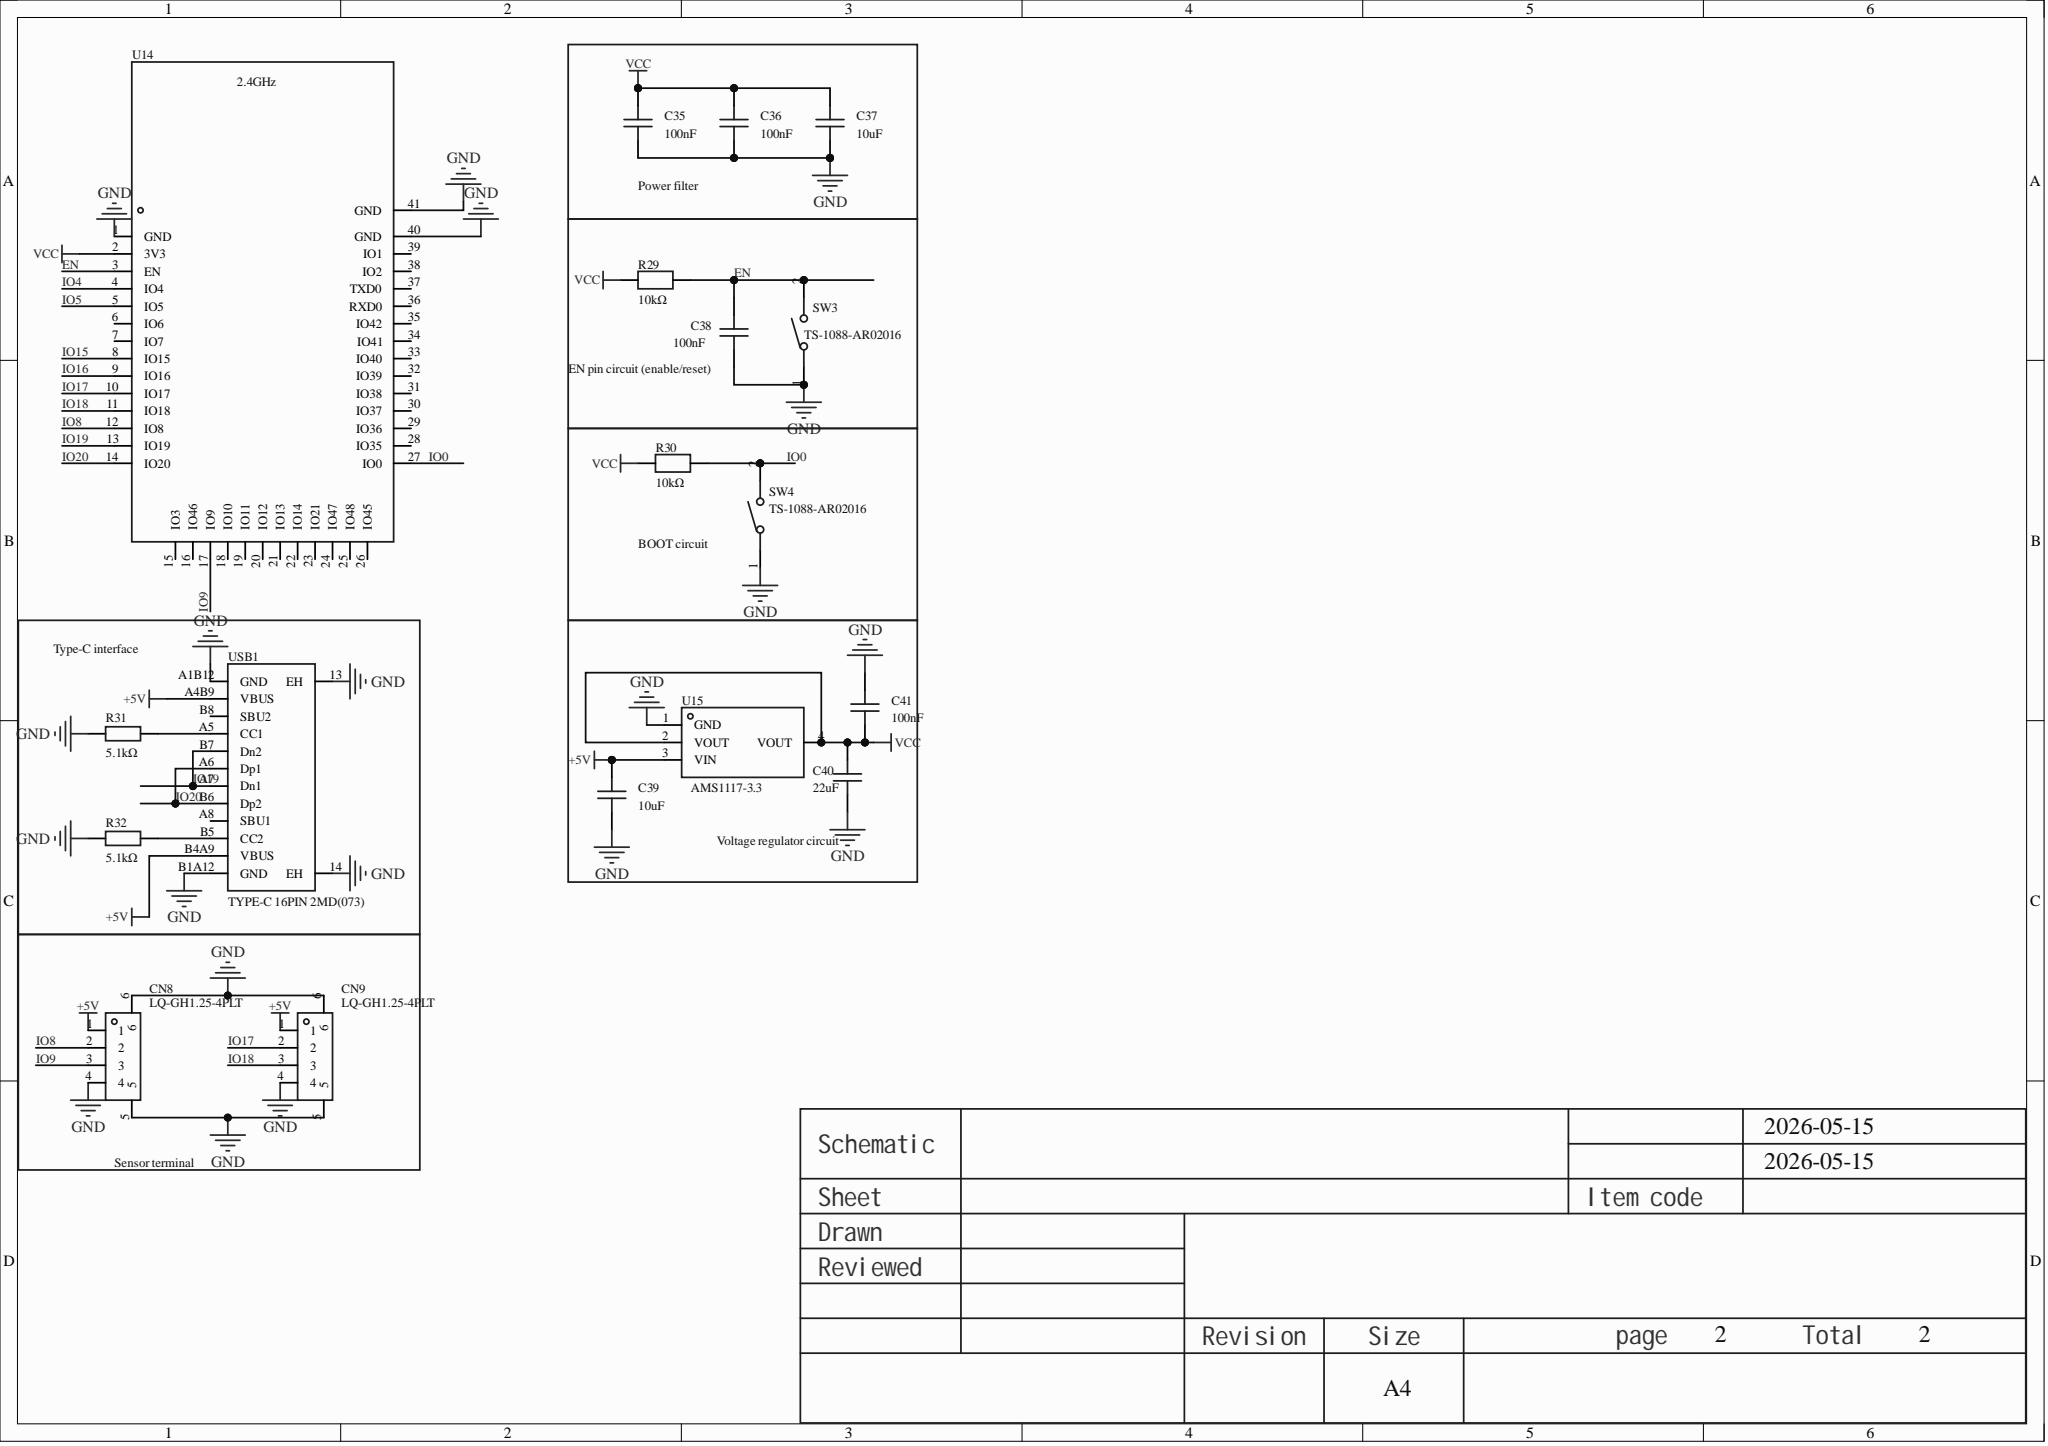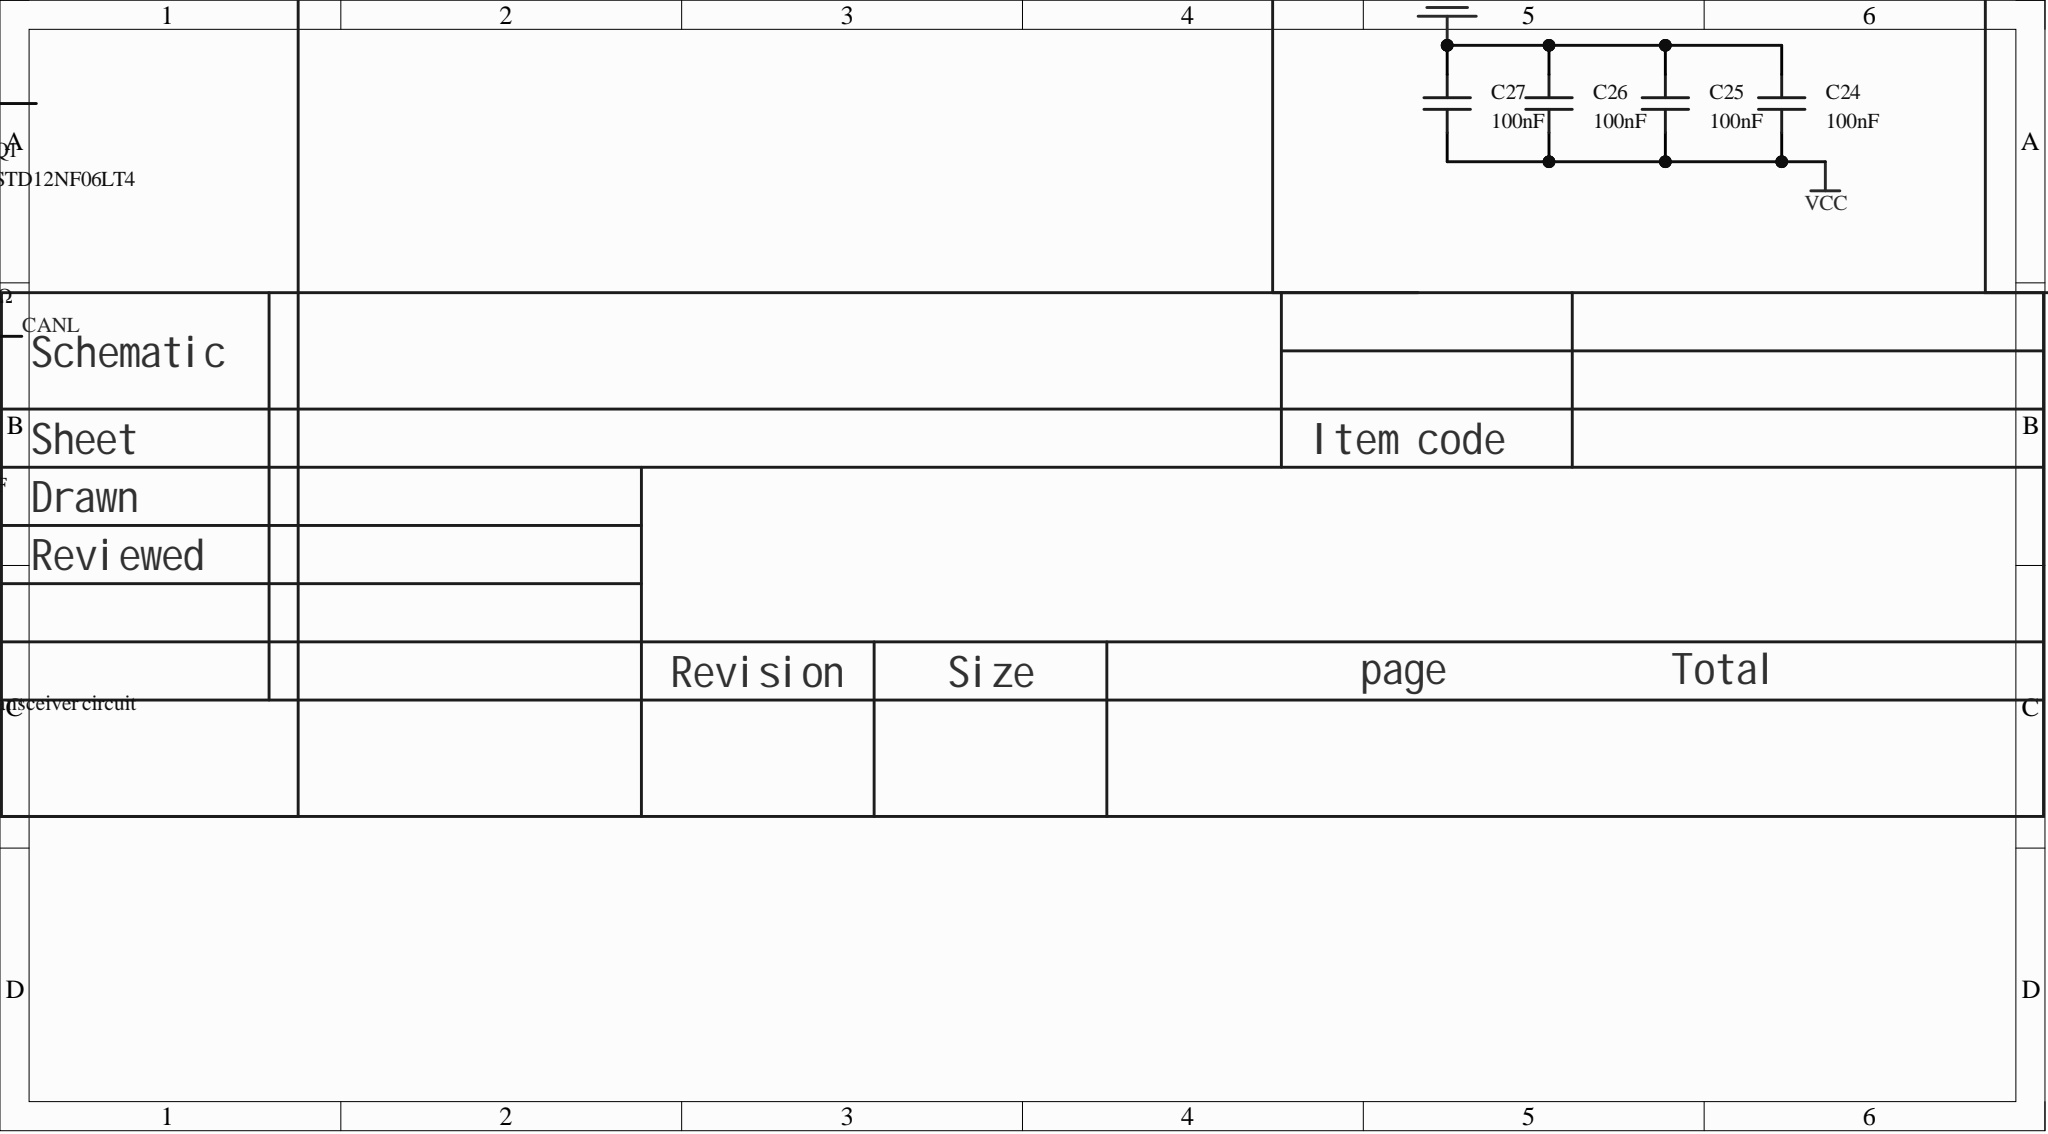Circuit board | Altium Designer | 106 parts | 73 nets
Bill of materials:
Comment,Description,Designator,Footprint,LibRef,Quantity
"CAPCER0.1UF16VX5R0603,CAPCER0.1UF25VX5R0603,CAPCER0.1UF16VX7R0603","","C1, C4, C9, C28","C0603","CAPCER0.1UF16VX5R0603,CAPCER0.1UF25VX5R0603,CAPCER0.1UF16VX7R0603","4"
"1uF","Capacitance: 1uF; Tolerance: ±10%; Rated voltage: 16V; Dielectric (temp coefficient): X7R;","C2, C3","C0603","GRM188R71C105KE15D","2"
"100nF","Capacitance: 100nF; Tolerance: ±10%; Rated voltage: 100V; Dielectric (temp coefficient): X7S;, Capacitance: 100nF; Tolerance: ±10%; Rated voltage: 50V; Temp coefficient: X7R;","C5, C6, C7, C8, C14, C15, C24, C25, C26, C27, C35, C36, C38, C41","C0603","C1608X7S2A104K080AE, CC0603KRX7R9BB104","14"
"18pF","Capacitance: 18pF; Tolerance: ±5%; Rated voltage: 50V; Dielectric (temp coefficient): C0G;","C10, C11, C29, C30","C0603","C1608C0G1H180J080AA","4"
"10uF","Capacitance: 10uF; Tolerance: ±10%; Rated voltage: 10V; Dielectric (temp coefficient): X5R;","C16","C0603","CL10A106KP8NNNC","1"
"22uF","Capacitance: 22uF; Tolerance: ±20%; Rated voltage: 6.3V; Dielectric (temp coefficient): X5R;","C17","C0603","CL10A226MQ8NRNC","1"
"30pF","Capacitance: 30pF; Tolerance: ±5%; Rated voltage: 50V; Dielectric (temp coefficient): NP0;","C18, C19, C33, C34","C0805","0805N300J500CT","4"
"10uF","Capacitance: 10uF; Tolerance: ±10%; Rated voltage: 50V; Temp coefficient: X5R;","C37, C39","C0805","CGA0805X5R106K500MT","2"
"22uF","Capacitance: 22uF; Tolerance: ±20%; Rated voltage: 35V; Temp coefficient: X5R;","C40","C0805","CGA0805X5R226M350MT","1"
"WAFER-GH1.25-3PLB","插针结构:1x3P;间距:1.25mm;安装方式:立贴;参考系列:GH;总PIN数:3P;排数:1;每排PIN数:3;额定电流:1A;工作温度范围:-25℃~+85℃;","CN1, CN2","CONN-SMD_3P-P1.25_XUNPU_WAFER-GH1.25-3PLB","WAFER-GH1.25-3PLB","2"
"2060-451/998-404","结构:1x1P;间距:-;颜色:白色;安装方式:-;总PIN数:1P;每排PIN数:1;排数:1;额定电流:9A;额定电压:600V;线规 - AWG:18~24;线规 - 平方毫米:-;工作温度:-60℃~+105℃;","CN3, CN10","CONN-SMD_L12.7-W3.9_2060-451-998-404","2060-451/998-404","2"
"WAFER-GH1.25-2PLB","插针结构:1x2P;间距:1.25mm;安装方式:立贴;参考系列:GH;总PIN数:2P;排数:1;每排PIN数:2;行距:-;额定电流:1A;触头材质:黄铜;触头镀层:-;工作温度范围:-25℃~+85℃;","CN4, CN5, CN6, CN7","CONN-TH_2P-P1.25_XUNPU_WAFER-GH1.25-2PLB","WAFER-GH1.25-2PLB","4"
"LQ-GH1.25-4PLT","1.25mm pitch 1x4P vertical-exit SMD wire-to-board header, suitable for SMT reflow","CN8, CN9","CONN-SMD_LQ-GH1.25-4PLT","LQ-GH1.25-4PLT","2"
"GH1.25-2P","插针结构:1x2P;间距:1.25mm;安装方式:立贴;参考系列:GH;总PIN数:2P;排数:1;每排PIN数:2;行距:-;额定电流:1A;触头材质:黄铜;触头镀层:-;工作温度范围:-25℃~+85℃;","CN11, CN12, CN13, CN14","CONN-TH_2P-P1.25_XUNPU_WAFER-GH1.25-2PLB","WAFER-GH1.25-2PLB","4"
"PZ254V-12-6P","插针结构:2x3P;间距:2.54mm;行距:2.54mm;圆针/方针:方针;安装类型:直插;排数:双排;总PIN位数:6P;额定电流:-;额定电压:-;配合针长度:6mm;塑高:2.5mm;端接针长度:3mm;触头材质:黄铜;触头镀层:-;工作温度范围:-40℃~+105℃;颜色:黑色;","H1, H3","HDR-TH_6P-P2.54-V-M-R2-C3-S2.54","PZ254V-12-6P","2"
"2541WR-04P","Pitch: 2.54mm; Mounting: right-angle THT; Rows: single; Mating pin length: 6mm; Plastic height: 2.54mm;","H2, H4","HDR-TH_4P-P2.54-H-M-W10.4-N","2541WR-04P","2"
"ME6211C33M5G-N","Output type: fixed; Max input voltage: 6V; Output voltage: 3.3V; Max output current: 500mA; PSRR: 70dB; Output polarity: positive;","LDO1","SOT-23-5_L3.0-W1.7-P0.95-LS2.8-BL","ME6211C33M5G-N","1"
"NCD0805R1","灯头类型:-;发光颜色:红色;正向电压(VF):1.6V~2.6V;功率:65mW;正向电流:20mA;主波长:615nm~630nm;二极管配置:独立二极管;透镜颜色:无色透明透镜;色温:-;发光强度:67mcd~195mcd;发光角度:130°;载带方式:-;工作温度:-30℃~+85℃;","PC13, PC14, PWR, PWR1","LED0805-R-RD","NCD0805R1","4"
"STD12NF06LT4","","Q1, Q2, Q3, Q4","TO-252-3_L6.5-W5.8-P4.58-BL","STD12NF06LT4","4"
"10kΩ","Resistor type: thick film resistor; Resistance: 10kΩ; Tolerance: ±1%; Power: 100mW; Max working voltage: 50V; Temp coefficient: ±100ppm/?;, Resistor type: thick film resistor; Resistance: 10kΩ; Tolerance: ±1%; Power: 100mW; Working voltage: 75V; Temp coefficient: ±100ppm/?;","R1, R2, R3, R4, R5, R6, R7, R11, R12, R13, R14, R15, R16, R17, R21, R22, R29, R30","R0603","ACD03K1002FT, FRC0603F1002TS","18"
"0Ω","Resistor type: thick film resistor; Resistance: 0Ω; Tolerance: ±1%;","R8, R9, R18, R19","R0805","RHC-05000FT","4"
"120Ω","Resistor type: thin film resistor; Resistance: 120Ω; Tolerance: ±1%; Power: 250mW; Max working voltage: 150V; Temp coefficient: ±25ppm/?;","R10, R20","R0805","TC0525F1200T5E","2"
"1kΩ","Resistor type: thick film resistor; Resistance: 1kΩ; Tolerance: ±1%; Power: 125mW; Max working voltage: 150V; Temp coefficient: ±100ppm/?;","R27, R28","R0805","0805W8F1001T5E","2"
"5.1kΩ","Resistor type: thick film resistor; Resistance: 5.1kΩ; Tolerance: ±1%; Power: 100mW; Working voltage: 75V; Temp coefficient: ±100ppm/?;","R31, R32","R0603","0603WAF5101T5E","2"
"TS-1101-C-W","电路结构:单刀单掷;按钮形状:矩形按钮;作用力:260gf;安装方式:立贴;开关长度:6mm;开关宽度:3.6mm;开关高度:2.5mm;带支架:不带;触点电流:50mA;额定电压(AC):-;额定电压(DC):12V;额定功率:-;绝缘电阻:-;带灯:无;机械寿命:5万次;","SW1, SW2","SW-SMD_L6.0-W3.3-LS8.0","TS-1101-C-W","2"
"TS-1088-AR02016","电路结构:单刀单掷;按钮形状:圆形按钮;作用力:1.6N;安装方式:立贴;开关长度:4mm;开关宽度:3mm;开关高度:2mm;带支架:不带支架;触点电流:50mA;额定电压:12V;工作寿命:10万次;","SW3, SW4","SW-SMD_L3.9-W3.0-P4.45","TS-1088-AR02016","2"
"SK12D07VG4","电路结构:单刀双掷;安装方式:-;额定电流(DC):500mA;额定电压(DC):50V;额定电流(AC):-;额定电压(AC):-;机械寿命:5千次;","SW5","SW-TH_SK12D07VG4","SK12D07VG4","1"
"STM32F103C8T6","CPU core: ARM-M3; Max CPU frequency: 72MHz; Application: -;","U1, U7","LQFP-48_L7.0-W7.0-P0.50-LS9.0-BL","STM32F103C8T6","2"
"0.1uF/100V","","U2, U9","C0805","0.1uF/100V_C9900010259","2"
"AMS1117-5.0","Output type: fixed; Max input voltage: 18V; Output voltage: 5V; Output current: 1A; PSRR: 70dB@(120Hz); Output polarity: positive;","U3","SOT-89-3_L4.5-W2.5-P1.50-LS4.2-BR","AMS1117-5.0","1"
"TJA1050T/CM-YJLTY","","U4, U8","SOIC-8_L4.9-W3.9-P1.27-LS6.0-BL","TJA1050T/CM-YJLTY","2"
"XT30U-F","Category: -; Type 1: -;","U6","CONN-TH_XT30U-F","XT30U-F","1"
"2.4GHz","Core chip: ESP32-S3R8; Frequency: 2.4GHz; Antenna: on-board PCB antenna; TX power: 20.5dBm; RX sensitivity: -103.5dBm;","U14","WIRELM-SMD_ESP32-S3-WROOM-1","ESP32-S3-WROOM-1-N16R8","1"
"AMS1117-3.3","Output type: fixed; Working voltage: 15V; Output voltage: 3.3V; Output current: 1A; PSRR: 72dB@(120Hz); Output polarity: positive;","U15","SOT-223-3_L6.5-W3.4-P2.30-LS7.0-BR","AMS1117-3.3_C6186","1"
"TYPE-C 16PIN 2MD(073)","Connector type: Type-C; Protocol standard: -; Gender: Female; Mounting: Flat SMD; Contacts: 16P; Ports: 1; Rated current - power: 3A; Operating temp: -25℃~+85℃;","USB1","USB-C-SMD_TYPE-C-16PIN-2MD-073","TYPE-C 16PIN 2MD(073)","1"
"8M crystal","","Y2, Y3","HC-49S_L11.5-W4.7-P4.88","8M晶振_C9900011272","2"
Netlist (Protel format):
[
C1
C0603
CAPCER0.1UF16VX5R0603,CAPCER0.1UF25VX5R0603,CAPCER0.1UF16VX7R0603



]
[
C2
C0603
1uF



]
[
C3
C0603
1uF



]
[
C4
C0603
CAPCER0.1UF16VX5R0603,CAPCER0.1UF25VX5R0603,CAPCER0.1UF16VX7R0603



]
[
C5
C0603
100nF



]
[
C6
C0603
100nF



]
[
C7
C0603
100nF



]
[
C8
C0603
100nF



]
[
C9
C0603
CAPCER0.1UF16VX5R0603,CAPCER0.1UF25VX5R0603,CAPCER0.1UF16VX7R0603



]
[
C10
C0603
18pF



]
[
C11
C0603
18pF



]
[
C14
C0603
100nF



]
[
C15
C0603
100nF



]
[
C16
C0603
10uF



]
[
C17
C0603
22uF



]
[
C18
C0805
30pF



]
[
C19
C0805
30pF



]
[
C24
C0603
100nF



]
[
C25
C0603
100nF



]
[
C26
C0603
100nF



]
[
C27
C0603
100nF



]
[
C28
C0603
CAPCER0.1UF16VX5R0603,CAPCER0.1UF25VX5R0603,CAPCER0.1UF16VX7R0603



]
[
C29
C0603
18pF



]
[
C30
C0603
18pF



]
[
C33
C0805
30pF



]
[
C34
C0805
30pF



]
[
C35
C0603
100nF



]
[
C36
C0603
100nF



]
[
C37
C0805
10uF



]
[
C38
C0603
100nF



]
[
C39
C0805
10uF



]
[
C40
C0805
22uF



]
[
C41
C0603
100nF



]
[
CN1
CONN-SMD_3P-P1.25_XUNPU_WAFER-GH1.25-3PLB
WAFER-GH1.25-3PLB



]
[
CN2
CONN-SMD_3P-P1.25_XUNPU_WAFER-GH1.25-3PLB
WAFER-GH1.25-3PLB



]
[
CN3
CONN-SMD_L12.7-W3.9_2060-451-998-404
2060-451/998-404



]
[
CN4
CONN-TH_2P-P1.25_XUNPU_WAFER-GH1.25-2PLB
WAFER-GH1.25-2PLB



]
[
CN5
CONN-TH_2P-P1.25_XUNPU_WAFER-GH1.25-2PLB
WAFER-GH1.25-2PLB



]
[
CN6
CONN-TH_2P-P1.25_XUNPU_WAFER-GH1.25-2PLB
WAFER-GH1.25-2PLB



]
[
CN7
CONN-TH_2P-P1.25_XUNPU_WAFER-GH1.25-2PLB
WAFER-GH1.25-2PLB



]
[
CN8
CONN-SMD_LQ-GH1.25-4PLT
LQ-GH1.25-4PLT



]
[
CN9
CONN-SMD_LQ-GH1.25-4PLT
LQ-GH1.25-4PLT



]
[
CN10
CONN-SMD_L12.7-W3.9_2060-451-998-404
2060-451/998-404



]
[
CN11
CONN-TH_2P-P1.25_XUNPU_WAFER-GH1.25-2PLB
GH1.25-2P



]
[
CN12
CONN-TH_2P-P1.25_XUNPU_WAFER-GH1.25-2PLB
GH1.25-2P



]
[
CN13
CONN-TH_2P-P1.25_XUNPU_WAFER-GH1.25-2PLB
GH1.25-2P



]
[
CN14
CONN-TH_2P-P1.25_XUNPU_WAFER-GH1.25-2PLB
GH1.25-2P



]
[
H1
HDR-TH_6P-P2.54-V-M-R2-C3-S2.54
PZ254V-12-6P



]
[
H2
HDR-TH_4P-P2.54-H-M-W10.4-N
2541WR-04P



]
[
H3
HDR-TH_6P-P2.54-V-M-R2-C3-S2.54
PZ254V-12-6P



]
[
H4
HDR-TH_4P-P2.54-H-M-W10.4-N
2541WR-04P



]
[
LDO1
SOT-23-5_L3.0-W1.7-P0.95-LS2.8-BL
ME6211C33M5G-N



]
[
PC13
LED0805-R-RD
NCD0805R1



]
[
PC14
LED0805-R-RD
NCD0805R1



]
[
PWR
LED0805-R-RD
NCD0805R1



]
[
PWR1
LED0805-R-RD
NCD0805R1



]
[
Q1
TO-252-3_L6.5-W5.8-P4.58-BL
STD12NF06LT4



]
[
Q2
TO-252-3_L6.5-W5.8-P4.58-BL
STD12NF06LT4



]
[
Q3
TO-252-3_L6.5-W5.8-P4.58-BL
STD12NF06LT4



]
[
Q4
TO-252-3_L6.5-W5.8-P4.58-BL
STD12NF06LT4



]
[
R1
R0603
10kΩ



]
[
R2
R0603
10kΩ



]
[
R3
R0603
10kΩ



]
[
R4
R0603
10kΩ



]
[
R5
R0603
10kΩ



]
[
R6
R0603
10kΩ



]
[
R7
R0603
10kΩ



]
[
R8
R0805
0Ω



]
[
R9
R0805
0Ω



]
[
R10
R0805
120Ω



]
[
R11
R0603
10kΩ



]
[
R12
R0603
10kΩ



]
[
R13
R0603
10kΩ



]
[
R14
R0603
10kΩ



]
[
R15
R0603
10kΩ



]
[
R16
R0603
10kΩ



]
[
R17
R0603
10kΩ



]
[
R18
R0805
0Ω



]
[
R19
R0805
0Ω



]
[
R20
R0805
120Ω



]
[
R21
R0603
10kΩ



]
[
R22
R0603
10kΩ



]
[
R27
R0805
1kΩ



]
[
R28
R0805
1kΩ



]
[
R29
R0603
10kΩ



]
[
R30
R0603
10kΩ



]
[
R31
R0603
5.1kΩ



]
[
R32
R0603
5.1kΩ



]
[
SW1
SW-SMD_L6.0-W3.3-LS8.0
TS-1101-C-W



]
[
SW2
SW-SMD_L6.0-W3.3-LS8.0
TS-1101-C-W



]
[
SW3
SW-SMD_L3.9-W3.0-P4.45
TS-1088-AR02016



]
[
SW4
SW-SMD_L3.9-W3.0-P4.45
TS-1088-AR02016



]
[
SW5
SW-TH_SK12D07VG4
SK12D07VG4



]
[
U1
LQFP-48_L7.0-W7.0-P0.50-LS9.0-BL
STM32F103C8T6



]
[
U2
C0805
0.1uF/100V



]
[
U3
SOT-89-3_L4.5-W2.5-P1.50-LS4.2-BR
AMS1117-5.0



]
[
U4
SOIC-8_L4.9-W3.9-P1.27-LS6.0-BL
TJA1050T/CM-YJLTY



]
[
U6
CONN-TH_XT30U-F
XT30U-F



]
[
U7
LQFP-48_L7.0-W7.0-P0.50-LS9.0-BL
STM32F103C8T6



]
[
U8
SOIC-8_L4.9-W3.9-P1.27-LS6.0-BL
TJA1050T/CM-YJLTY



]
[
U9
C0805
0.1uF/100V



]
[
U14
WIRELM-SMD_ESP32-S3-WROOM-1
2.4GHz



]
[
U15
SOT-223-3_L6.5-W3.4-P2.30-LS7.0-BR
AMS1117-3.3



]
[
USB1
USB-C-SMD_TYPE-C-16PIN-2MD-073
TYPE-C 16PIN 2MD(073)



]
[
Y2
HC-49S_L11.5-W4.7-P4.88
8M crystal



]
[
Y3
HC-49S_L11.5-W4.7-P4.88
8M crystal



]
(
VCC
C3-2
C4-2
C5-2
C6-2
C7-2
C8-2
C24-2
C25-2
C26-2
C27-2
C35-2
C36-2
C37-2
C40-2
C41-1
H1-1
H1-2
H2-1
H3-1
H3-2
H4-1
LDO1-5
PC13-1
PC14-1
PWR-1
PWR1-1
R5-2
R7-2
R15-2
R17-2
R29-1
R30-1
U1-9
U1-24
U1-36
U1-48
U7-9
U7-24
U7-36
U7-48
U14-2
U15-2
U15-4
)
(
SWIOB
H4-2
R15-1
U7-34
)
(
SWIO
H2-2
R5-1
U1-34
)
(
SWCLKB
H4-3
R16-2
U7-37
)
(
SWCLK
H2-3
R6-2
U1-37
)
(
RESETB
C28-2
R17-1
SW2-1
U7-7
)
(
RESET
C9-2
R7-1
SW1-1
U1-7
)
(
POWER
SW5-1
U6-2
)
(
PC13B
R12-2
U7-2
)
(
PC13
R2-2
U1-2
)
(
PA12B
U7-33
U8-1
)
(
PA12
U1-33
U4-1
)
(
PA11B
U7-32
U8-4
)
(
PA11
U1-32
U4-4
)
(
PA10B
CN7-2
U7-31
)
(
PA10
CN6-2
U1-31
)
(
PA9B
CN7-1
U7-30
)
(
PA9
CN6-1
U1-30
)
(
PA8B
Q4-1
U7-29
)
(
PA8
Q3-1
U1-29
)
(
PA6B
CN2-1
U7-16
)
(
PA6
CN1-1
U1-16
)
(
PA3B
CN5-2
U7-13
)
(
PA3
CN4-2
U1-13
)
(
PA2B
CN5-1
U7-12
)
(
PA2
CN4-1
U1-12
)
(
OUTPUT
C14-2
C16-2
CN1-2
CN2-2
R27-2
R28-2
SW5-2
U3-3
)
(
OSOUTB
C30-1
U7-6
Y3-2
)
(
OSOUT
C11-1
U1-6
Y2-2
)
(
OSCINB
C29-1
U7-5
Y3-1
)
(
OSCIN
C10-1
U1-5
Y2-1
)
(
NetR32_2
R32-2
USB1-B5
)
(
NetR31_2
R31-2
USB1-A5
)
(
NetR22_2
R22-2
U8-5
)
(
NetR21_2
R21-2
U4-5
)
(
NetR19_1
R19-1
U8-6
)
(
NetR18_1
R18-1
U8-7
)
(
NetR9_1
R9-1
U4-6
)
(
NetR8_1
R8-1
U4-7
)
(
NetQ2_3
Q2-3
R20-2
)
(
NetQ2_1
Q2-1
Q4-2
R28-1
)
(
NetQ1_3
Q1-3
R10-2
)
(
NetQ1_1
Q1-1
Q3-2
R27-1
)
(
NetPWR_2
PWR-2
R1-1
)
(
NetPWR1_2
PWR1-2
R11-1
)
(
NetPC14_2
PC14-2
R12-1
)
(
NetPC13_2
PC13-2
R2-1
)
(
NetH3_4
H3-4
R14-1
)
(
NetH3_3
H3-3
R13-2
)
(
NetH1_4
H1-4
R4-1
)
(
NetH1_3
H1-3
R3-2
)
(
IO20
U14-14
USB1-A6
USB1-B6
)
(
IO19
U14-13
USB1-A7
USB1-B7
)
(
IO18
CN9-3
U14-11
)
(
IO17
CN9-2
U14-10
)
(
IO16
U7-21
U14-9
)
(
IO15
U7-22
U14-8
)
(
IO9
CN8-3
U14-17
)
(
IO8
CN8-2
U14-12
)
(
IO5
U1-21
U14-5
)
(
IO4
U1-22
U14-4
)
(
IO0
R30-2
SW4-2
U14-27
)
(
GND
C1-1
C2-1
C3-1
C4-1
C5-1
C6-1
C7-1
C8-1
C9-1
C10-2
C11-2
C14-1
C15-2
C16-1
C17-2
C18-1
C19-1
C24-1
C25-1
C26-1
C27-1
C28-1
C29-2
C30-2
C33-1
C34-1
C35-1
C36-1
C37-1
C38-1
C39-1
C40-1
C41-2
CN1-3
CN1-4
CN1-5
CN2-3
CN2-4
CN2-5
CN3-1
CN3-2
CN4-3
CN4-4
CN5-3
CN5-4
CN6-3
CN6-4
CN7-3
CN7-4
CN8-4
CN8-5
CN8-6
CN9-4
CN9-5
CN9-6
CN10-1
CN10-2
CN11-3
CN11-4
CN12-3
CN12-4
CN13-3
CN13-4
CN14-3
CN14-4
H1-5
H1-6
H2-4
H3-5
H3-6
H4-4
LDO1-2
Q3-3
Q4-3
R1-2
R6-1
R11-2
R16-1
R21-1
R22-1
R31-1
R32-1
SW1-2
SW2-2
SW3-1
SW4-1
SW5-4
SW5-5
U1-1
U1-8
U1-23
U1-35
U1-47
U2-2
U3-1
U4-2
U4-8
U6-1
U7-1
U7-8
U7-23
U7-35
U7-47
U8-2
U8-8
U9-2
U14-1
U14-40
U14-41
U15-1
USB1-13
USB1-14
USB1-A1B12
USB1-B1A12
)
(
EN
C38-2
R29-2
SW3-2
U14-3
)
(
CANLB
C34-2
CN13-1
CN14-1
R19-2
R20-1
)
(
CANL
C19-2
CN11-1
CN12-1
R9-2
R10-1
)
(
CANHB
C33-2
CN13-2
CN14-2
Q2-2
R18-2
)
(
CANH
C18-2
CN11-2
CN12-2
Q1-2
R8-2
)
(
BOOT1B
R14-2
U7-20
)
(
BOOT1
R4-2
U1-20
)
(
BOOT0B
R13-1
U7-44
)
(
BOOT0
R3-1
U1-44
)
(
+5V
C1-2
C2-2
C15-1
C17-1
C39-2
CN8-1
CN9-1
LDO1-1
LDO1-3
U2-1
U3-2
U4-3
U8-3
U9-1
U15-3
USB1-A4B9
USB1-B4A9
)